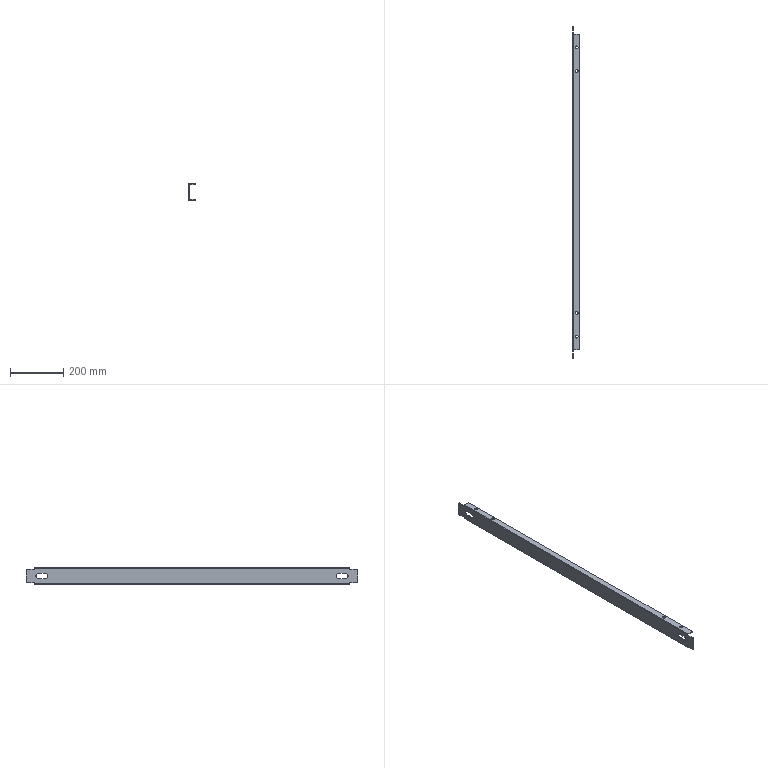Part | SolidWorks | features SMBaseFlange 2, Cut 1, Fillet 1, FlatPattern 1, ICE 1, SheetMetal 1 | 1 solid | 58 faces | box 25 x 1249 x 62 mm | volume 374837 mm3 | plane 30 | cylinder 28 | commonest cylinder face diameters 11 x16 6 x4 20 x4 0.4 x2 6.4 x2